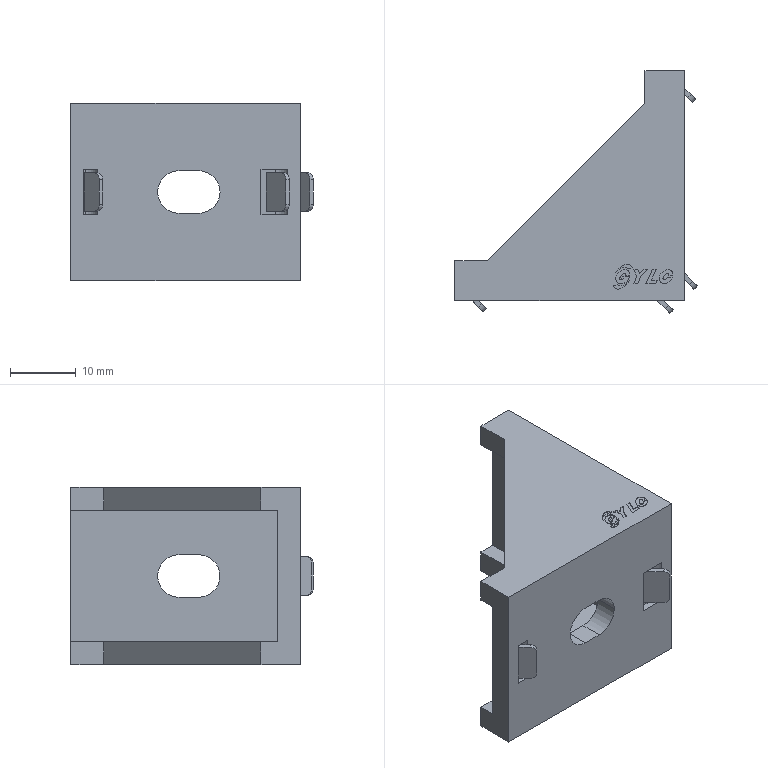Part | SolidWorks | features ICE 7, Fillet 3, MirrorPattern 2, Extrusion 1, Shell 1 | 1 solid | 125 faces | box 36.96 x 36.96 x 27 mm | volume 8976 mm3 | plane 90 | spline 18 | cylinder 17 | commonest cylinder face diameters 2 x8 6.5 x5 4 x4